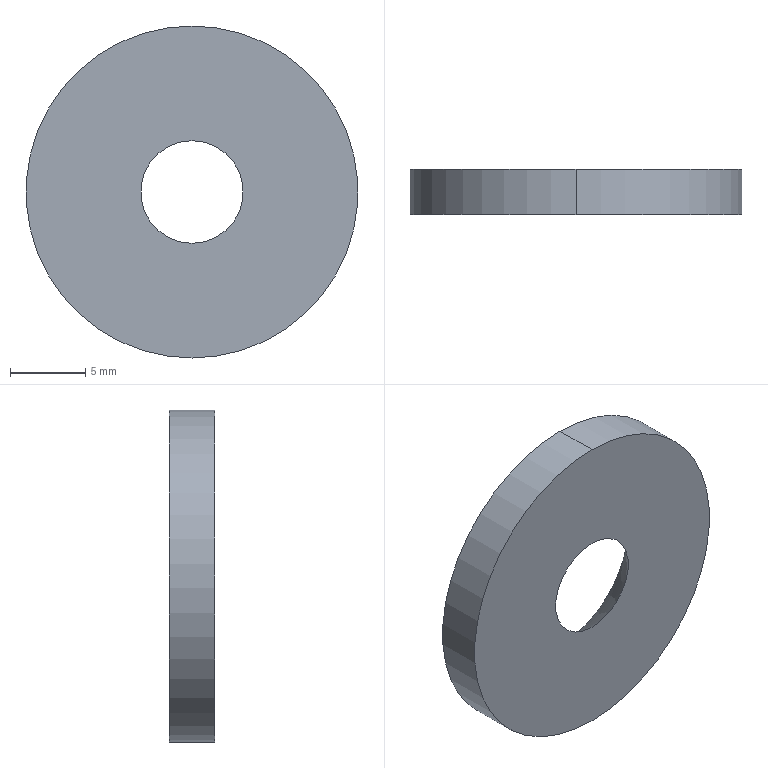Part | SolidWorks | features FlatPattern 1, HoleWzd 1, SMBaseFlange 1, SheetMetal 1 | 1 solid | 6 faces | box 22 x 3 x 22 mm | volume 907.041 mm3 | cone 2 | cylinder 2 | plane 2 | commonest cylinder face diameters 22 x2
STEP:
#1=CARTESIAN_POINT('',(0.,-3.,-3.4));
#2=VERTEX_POINT('',#1);
#3=CARTESIAN_POINT('',(0.,-3.,3.4));
#4=VERTEX_POINT('',#3);
#5=CARTESIAN_POINT('',(0.,-3.,0.));
#6=DIRECTION('',(0.,1.,0.));
#7=DIRECTION('',(0.,0.,1.));
#8=AXIS2_PLACEMENT_3D('',#5,#6,#7);
#9=CIRCLE('',#8,3.4);
#10=EDGE_CURVE('',#2,#4,#9,.T.);
#11=ORIENTED_EDGE('',*,*,#10,.F.);
#12=CARTESIAN_POINT('',(0.,0.,-6.4));
#13=VERTEX_POINT('',#12);
#14=CARTESIAN_POINT('',(0.,0.,-6.4));
#15=DIRECTION('',(0.,0.7071,-0.7071));
#16=VECTOR('',#15,1000.);
#17=LINE('',#14,#16);
#18=EDGE_CURVE('',#2,#13,#17,.T.);
#19=ORIENTED_EDGE('',*,*,#18,.T.);
#20=CARTESIAN_POINT('',(0.,0.,6.4));
#21=VERTEX_POINT('',#20);
#22=CARTESIAN_POINT('',(0.,0.,0.));
#23=DIRECTION('',(0.,1.,0.));
#24=DIRECTION('',(0.,0.,1.));
#25=AXIS2_PLACEMENT_3D('',#22,#23,#24);
#26=CIRCLE('',#25,6.4);
#27=EDGE_CURVE('',#13,#21,#26,.T.);
#28=ORIENTED_EDGE('',*,*,#27,.T.);
#29=CARTESIAN_POINT('',(0.,0.,6.4));
#30=DIRECTION('',(0.,0.7071,0.7071));
#31=VECTOR('',#30,1000.);
#32=LINE('',#29,#31);
#33=EDGE_CURVE('',#4,#21,#32,.T.);
#34=ORIENTED_EDGE('',*,*,#33,.F.);
#35=EDGE_LOOP('',(#11,#19,#28,#34));
#36=FACE_OUTER_BOUND('',#35,.T.);
#37=CARTESIAN_POINT('',(0.,0.,0.));
#38=DIRECTION('',(0.,1.,0.));
#39=DIRECTION('',(0.,0.,1.));
#40=AXIS2_PLACEMENT_3D('',#37,#38,#39);
#41=CONICAL_SURFACE('',#40,6.4,0.7854);
#42=ADVANCED_FACE('',(#36),#41,.F.);
#43=CARTESIAN_POINT('',(0.,-3.,11.));
#44=VERTEX_POINT('',#43);
#45=CARTESIAN_POINT('',(0.,-3.,-11.));
#46=VERTEX_POINT('',#45);
#47=CARTESIAN_POINT('',(0.,-3.,0.));
#48=DIRECTION('',(0.,1.,0.));
#49=DIRECTION('',(0.,0.,1.));
#50=AXIS2_PLACEMENT_3D('',#47,#48,#49);
#51=CIRCLE('',#50,11.);
#52=EDGE_CURVE('',#44,#46,#51,.T.);
#53=ORIENTED_EDGE('',*,*,#52,.T.);
#54=CARTESIAN_POINT('',(0.,0.,-11.));
#55=VERTEX_POINT('',#54);
#56=CARTESIAN_POINT('',(0.,-3.,-11.));
#57=DIRECTION('',(0.,1.,0.));
#58=VECTOR('',#57,1000.);
#59=LINE('',#56,#58);
#60=EDGE_CURVE('',#46,#55,#59,.T.);
#61=ORIENTED_EDGE('',*,*,#60,.T.);
#62=CARTESIAN_POINT('',(0.,0.,11.));
#63=VERTEX_POINT('',#62);
#64=CARTESIAN_POINT('',(0.,0.,0.));
#65=DIRECTION('',(0.,1.,0.));
#66=DIRECTION('',(0.,0.,1.));
#67=AXIS2_PLACEMENT_3D('',#64,#65,#66);
#68=CIRCLE('',#67,11.);
#69=EDGE_CURVE('',#63,#55,#68,.T.);
#70=ORIENTED_EDGE('',*,*,#69,.F.);
#71=CARTESIAN_POINT('',(0.,-3.,11.));
#72=DIRECTION('',(0.,1.,0.));
#73=VECTOR('',#72,1000.);
#74=LINE('',#71,#73);
#75=EDGE_CURVE('',#44,#63,#74,.T.);
#76=ORIENTED_EDGE('',*,*,#75,.F.);
#77=EDGE_LOOP('',(#53,#61,#70,#76));
#78=FACE_OUTER_BOUND('',#77,.T.);
#79=CARTESIAN_POINT('',(0.,-3.,0.));
#80=DIRECTION('',(0.,1.,0.));
#81=DIRECTION('',(0.,0.,1.));
#82=AXIS2_PLACEMENT_3D('',#79,#80,#81);
#83=CYLINDRICAL_SURFACE('',#82,11.);
#84=ADVANCED_FACE('',(#78),#83,.T.);
#85=ORIENTED_EDGE('',*,*,#60,.F.);
#86=CARTESIAN_POINT('',(0.,-3.,0.));
#87=DIRECTION('',(0.,1.,0.));
#88=DIRECTION('',(0.,0.,1.));
#89=AXIS2_PLACEMENT_3D('',#86,#87,#88);
#90=CIRCLE('',#89,11.);
#91=EDGE_CURVE('',#46,#44,#90,.T.);
#92=ORIENTED_EDGE('',*,*,#91,.T.);
#93=ORIENTED_EDGE('',*,*,#75,.T.);
#94=CARTESIAN_POINT('',(0.,0.,0.));
#95=DIRECTION('',(0.,1.,0.));
#96=DIRECTION('',(0.,0.,1.));
#97=AXIS2_PLACEMENT_3D('',#94,#95,#96);
#98=CIRCLE('',#97,11.);
#99=EDGE_CURVE('',#55,#63,#98,.T.);
#100=ORIENTED_EDGE('',*,*,#99,.F.);
#101=EDGE_LOOP('',(#85,#92,#93,#100));
#102=FACE_OUTER_BOUND('',#101,.T.);
#103=CARTESIAN_POINT('',(0.,-3.,0.));
#104=DIRECTION('',(0.,1.,0.));
#105=DIRECTION('',(0.,0.,1.));
#106=AXIS2_PLACEMENT_3D('',#103,#104,#105);
#107=CYLINDRICAL_SURFACE('',#106,11.);
#108=ADVANCED_FACE('',(#102),#107,.T.);
#109=CARTESIAN_POINT('',(0.,-3.,0.));
#110=DIRECTION('',(0.,1.,0.));
#111=DIRECTION('',(0.,0.,1.));
#112=AXIS2_PLACEMENT_3D('',#109,#110,#111);
#113=CIRCLE('',#112,3.4);
#114=EDGE_CURVE('',#4,#2,#113,.T.);
#115=ORIENTED_EDGE('',*,*,#114,.T.);
#116=ORIENTED_EDGE('',*,*,#10,.T.);
#117=EDGE_LOOP('',(#115,#116));
#118=FACE_BOUND('',#117,.T.);
#119=ORIENTED_EDGE('',*,*,#52,.F.);
#120=ORIENTED_EDGE('',*,*,#91,.F.);
#121=EDGE_LOOP('',(#119,#120));
#122=FACE_OUTER_BOUND('',#121,.T.);
#123=CARTESIAN_POINT('',(0.,-3.,0.));
#124=DIRECTION('',(0.,1.,0.));
#125=DIRECTION('',(0.,0.,1.));
#126=AXIS2_PLACEMENT_3D('',#123,#124,#125);
#127=PLANE('',#126);
#128=ADVANCED_FACE('',(#118,#122),#127,.F.);
#129=CARTESIAN_POINT('',(0.,0.,0.));
#130=DIRECTION('',(0.,1.,0.));
#131=DIRECTION('',(0.,0.,1.));
#132=AXIS2_PLACEMENT_3D('',#129,#130,#131);
#133=CIRCLE('',#132,6.4);
#134=EDGE_CURVE('',#21,#13,#133,.T.);
#135=ORIENTED_EDGE('',*,*,#134,.F.);
#136=ORIENTED_EDGE('',*,*,#27,.F.);
#137=EDGE_LOOP('',(#135,#136));
#138=FACE_BOUND('',#137,.T.);
#139=ORIENTED_EDGE('',*,*,#69,.T.);
#140=ORIENTED_EDGE('',*,*,#99,.T.);
#141=EDGE_LOOP('',(#139,#140));
#142=FACE_OUTER_BOUND('',#141,.T.);
#143=CARTESIAN_POINT('',(0.,0.,0.));
#144=DIRECTION('',(0.,1.,0.));
#145=DIRECTION('',(0.,0.,1.));
#146=AXIS2_PLACEMENT_3D('',#143,#144,#145);
#147=PLANE('',#146);
#148=ADVANCED_FACE('',(#138,#142),#147,.T.);
#149=ORIENTED_EDGE('',*,*,#18,.F.);
#150=ORIENTED_EDGE('',*,*,#114,.F.);
#151=ORIENTED_EDGE('',*,*,#33,.T.);
#152=ORIENTED_EDGE('',*,*,#134,.T.);
#153=EDGE_LOOP('',(#149,#150,#151,#152));
#154=FACE_OUTER_BOUND('',#153,.T.);
#155=CARTESIAN_POINT('',(0.,0.,0.));
#156=DIRECTION('',(0.,1.,0.));
#157=DIRECTION('',(0.,0.,1.));
#158=AXIS2_PLACEMENT_3D('',#155,#156,#157);
#159=CONICAL_SURFACE('',#158,6.4,0.7854);
#160=ADVANCED_FACE('',(#154),#159,.F.);
#161=CLOSED_SHELL('',(#42,#84,#108,#128,#148,#160));
#162=MANIFOLD_SOLID_BREP('',#161);
#163=CARTESIAN_POINT('',(0.,0.,0.));
#164=DIRECTION('',(0.,0.,1.));
#165=DIRECTION('',(1.,0.,0.));
#166=AXIS2_PLACEMENT_3D('',#163,#164,#165);
#167=(LENGTH_UNIT()NAMED_UNIT(*)SI_UNIT(.MILLI.,.METRE.));
#168=UNCERTAINTY_MEASURE_WITH_UNIT(LENGTH_MEASURE(0.00001),#167,'','');
#169=(NAMED_UNIT(*)PLANE_ANGLE_UNIT()SI_UNIT($,.RADIAN.));
#170=(NAMED_UNIT(*)SI_UNIT($,.STERADIAN.)SOLID_ANGLE_UNIT());
#171=(GEOMETRIC_REPRESENTATION_CONTEXT(3)GLOBAL_UNCERTAINTY_ASSIGNED_CONTEXT((#168))GLOBAL_UNIT_ASSIGNED_CONTEXT((#167,#169,#170))REPRESENTATION_CONTEXT('',''));
#172=ADVANCED_BREP_SHAPE_REPRESENTATION('',(#162,#166),#171);